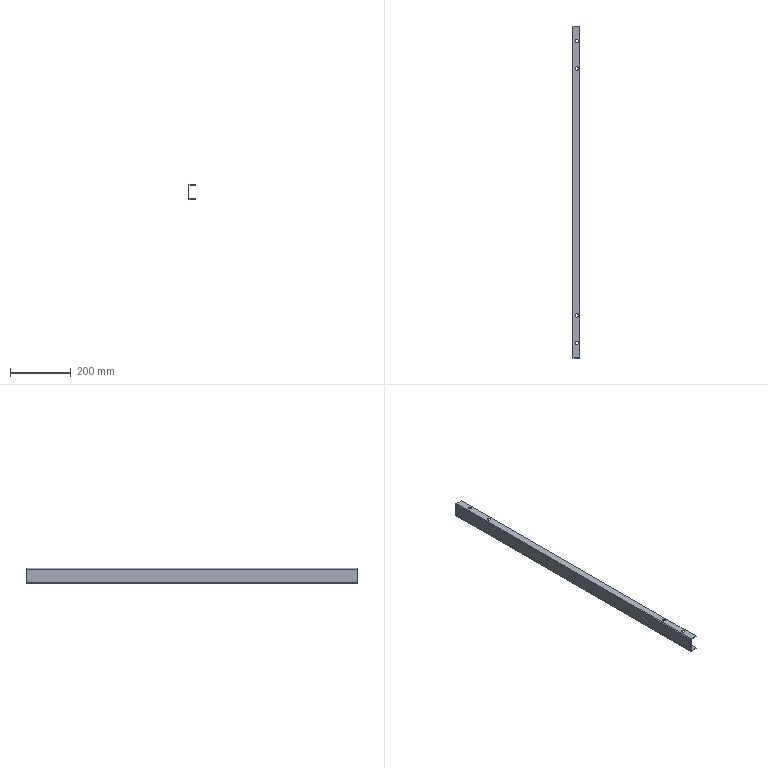Part | SolidWorks | features FlatPattern 1, ICE 1, SMBaseFlange 1, SheetMetal 1 | 1 solid | 38 faces | box 25 x 1095 x 50 mm | volume 206464 mm3 | cylinder 20 | plane 18 | commonest cylinder face diameters 11 x16 0.4 x2 4.4 x2
STEP:
#1=CARTESIAN_POINT('',(20.5,497.5,-23.));
#2=VERTEX_POINT('',#1);
#3=CARTESIAN_POINT('',(9.5,497.5,-23.));
#4=VERTEX_POINT('',#3);
#5=CARTESIAN_POINT('',(15.,497.5,-23.));
#6=DIRECTION('',(0.,0.,-1.));
#7=DIRECTION('',(-1.,0.,0.));
#8=AXIS2_PLACEMENT_3D('',#5,#6,#7);
#9=CIRCLE('',#8,5.5);
#10=EDGE_CURVE('',#2,#4,#9,.T.);
#11=ORIENTED_EDGE('',*,*,#10,.F.);
#12=CARTESIAN_POINT('',(20.5,497.5,-25.));
#13=VERTEX_POINT('',#12);
#14=CARTESIAN_POINT('',(20.5,497.5,25.));
#15=DIRECTION('',(0.,0.,-1.));
#16=VECTOR('',#15,1000.);
#17=LINE('',#14,#16);
#18=EDGE_CURVE('',#2,#13,#17,.T.);
#19=ORIENTED_EDGE('',*,*,#18,.T.);
#20=CARTESIAN_POINT('',(9.5,497.5,-25.));
#21=VERTEX_POINT('',#20);
#22=CARTESIAN_POINT('',(15.,497.5,-25.));
#23=DIRECTION('',(0.,0.,-1.));
#24=DIRECTION('',(-1.,0.,0.));
#25=AXIS2_PLACEMENT_3D('',#22,#23,#24);
#26=CIRCLE('',#25,5.5);
#27=EDGE_CURVE('',#13,#21,#26,.T.);
#28=ORIENTED_EDGE('',*,*,#27,.T.);
#29=CARTESIAN_POINT('',(9.5,497.5,25.));
#30=DIRECTION('',(0.,0.,-1.));
#31=VECTOR('',#30,1000.);
#32=LINE('',#29,#31);
#33=EDGE_CURVE('',#4,#21,#32,.T.);
#34=ORIENTED_EDGE('',*,*,#33,.F.);
#35=EDGE_LOOP('',(#11,#19,#28,#34));
#36=FACE_OUTER_BOUND('',#35,.T.);
#37=CARTESIAN_POINT('',(15.,497.5,25.));
#38=DIRECTION('',(0.,0.,-1.));
#39=DIRECTION('',(-1.,0.,0.));
#40=AXIS2_PLACEMENT_3D('',#37,#38,#39);
#41=CYLINDRICAL_SURFACE('',#40,5.5);
#42=ADVANCED_FACE('',(#36),#41,.F.);
#43=CARTESIAN_POINT('',(20.5,407.5,-23.));
#44=VERTEX_POINT('',#43);
#45=CARTESIAN_POINT('',(9.5,407.5,-23.));
#46=VERTEX_POINT('',#45);
#47=CARTESIAN_POINT('',(15.,407.5,-23.));
#48=DIRECTION('',(0.,0.,-1.));
#49=DIRECTION('',(-1.,0.,0.));
#50=AXIS2_PLACEMENT_3D('',#47,#48,#49);
#51=CIRCLE('',#50,5.5);
#52=EDGE_CURVE('',#44,#46,#51,.T.);
#53=ORIENTED_EDGE('',*,*,#52,.F.);
#54=CARTESIAN_POINT('',(20.5,407.5,-25.));
#55=VERTEX_POINT('',#54);
#56=CARTESIAN_POINT('',(20.5,407.5,25.));
#57=DIRECTION('',(0.,0.,-1.));
#58=VECTOR('',#57,1000.);
#59=LINE('',#56,#58);
#60=EDGE_CURVE('',#44,#55,#59,.T.);
#61=ORIENTED_EDGE('',*,*,#60,.T.);
#62=CARTESIAN_POINT('',(9.5,407.5,-25.));
#63=VERTEX_POINT('',#62);
#64=CARTESIAN_POINT('',(15.,407.5,-25.));
#65=DIRECTION('',(0.,0.,-1.));
#66=DIRECTION('',(-1.,0.,0.));
#67=AXIS2_PLACEMENT_3D('',#64,#65,#66);
#68=CIRCLE('',#67,5.5);
#69=EDGE_CURVE('',#55,#63,#68,.T.);
#70=ORIENTED_EDGE('',*,*,#69,.T.);
#71=CARTESIAN_POINT('',(9.5,407.5,25.));
#72=DIRECTION('',(0.,0.,-1.));
#73=VECTOR('',#72,1000.);
#74=LINE('',#71,#73);
#75=EDGE_CURVE('',#46,#63,#74,.T.);
#76=ORIENTED_EDGE('',*,*,#75,.F.);
#77=EDGE_LOOP('',(#53,#61,#70,#76));
#78=FACE_OUTER_BOUND('',#77,.T.);
#79=CARTESIAN_POINT('',(15.,407.5,25.));
#80=DIRECTION('',(0.,0.,-1.));
#81=DIRECTION('',(-1.,0.,0.));
#82=AXIS2_PLACEMENT_3D('',#79,#80,#81);
#83=CYLINDRICAL_SURFACE('',#82,5.5);
#84=ADVANCED_FACE('',(#78),#83,.F.);
#85=CARTESIAN_POINT('',(20.5,-407.5,-23.));
#86=VERTEX_POINT('',#85);
#87=CARTESIAN_POINT('',(9.5,-407.5,-23.));
#88=VERTEX_POINT('',#87);
#89=CARTESIAN_POINT('',(15.,-407.5,-23.));
#90=DIRECTION('',(0.,0.,-1.));
#91=DIRECTION('',(-1.,0.,0.));
#92=AXIS2_PLACEMENT_3D('',#89,#90,#91);
#93=CIRCLE('',#92,5.5);
#94=EDGE_CURVE('',#86,#88,#93,.T.);
#95=ORIENTED_EDGE('',*,*,#94,.F.);
#96=CARTESIAN_POINT('',(20.5,-407.5,-25.));
#97=VERTEX_POINT('',#96);
#98=CARTESIAN_POINT('',(20.5,-407.5,25.));
#99=DIRECTION('',(0.,0.,-1.));
#100=VECTOR('',#99,1000.);
#101=LINE('',#98,#100);
#102=EDGE_CURVE('',#86,#97,#101,.T.);
#103=ORIENTED_EDGE('',*,*,#102,.T.);
#104=CARTESIAN_POINT('',(9.5,-407.5,-25.));
#105=VERTEX_POINT('',#104);
#106=CARTESIAN_POINT('',(15.,-407.5,-25.));
#107=DIRECTION('',(0.,0.,-1.));
#108=DIRECTION('',(-1.,0.,0.));
#109=AXIS2_PLACEMENT_3D('',#106,#107,#108);
#110=CIRCLE('',#109,5.5);
#111=EDGE_CURVE('',#97,#105,#110,.T.);
#112=ORIENTED_EDGE('',*,*,#111,.T.);
#113=CARTESIAN_POINT('',(9.5,-407.5,25.));
#114=DIRECTION('',(0.,0.,-1.));
#115=VECTOR('',#114,1000.);
#116=LINE('',#113,#115);
#117=EDGE_CURVE('',#88,#105,#116,.T.);
#118=ORIENTED_EDGE('',*,*,#117,.F.);
#119=EDGE_LOOP('',(#95,#103,#112,#118));
#120=FACE_OUTER_BOUND('',#119,.T.);
#121=CARTESIAN_POINT('',(15.,-407.5,25.));
#122=DIRECTION('',(0.,0.,-1.));
#123=DIRECTION('',(-1.,0.,0.));
#124=AXIS2_PLACEMENT_3D('',#121,#122,#123);
#125=CYLINDRICAL_SURFACE('',#124,5.5);
#126=ADVANCED_FACE('',(#120),#125,.F.);
#127=CARTESIAN_POINT('',(20.5,-497.5,-23.));
#128=VERTEX_POINT('',#127);
#129=CARTESIAN_POINT('',(9.5,-497.5,-23.));
#130=VERTEX_POINT('',#129);
#131=CARTESIAN_POINT('',(15.,-497.5,-23.));
#132=DIRECTION('',(0.,0.,-1.));
#133=DIRECTION('',(-1.,0.,0.));
#134=AXIS2_PLACEMENT_3D('',#131,#132,#133);
#135=CIRCLE('',#134,5.5);
#136=EDGE_CURVE('',#128,#130,#135,.T.);
#137=ORIENTED_EDGE('',*,*,#136,.F.);
#138=CARTESIAN_POINT('',(20.5,-497.5,-25.));
#139=VERTEX_POINT('',#138);
#140=CARTESIAN_POINT('',(20.5,-497.5,25.));
#141=DIRECTION('',(0.,0.,-1.));
#142=VECTOR('',#141,1000.);
#143=LINE('',#140,#142);
#144=EDGE_CURVE('',#128,#139,#143,.T.);
#145=ORIENTED_EDGE('',*,*,#144,.T.);
#146=CARTESIAN_POINT('',(9.5,-497.5,-25.));
#147=VERTEX_POINT('',#146);
#148=CARTESIAN_POINT('',(15.,-497.5,-25.));
#149=DIRECTION('',(0.,0.,-1.));
#150=DIRECTION('',(-1.,0.,0.));
#151=AXIS2_PLACEMENT_3D('',#148,#149,#150);
#152=CIRCLE('',#151,5.5);
#153=EDGE_CURVE('',#139,#147,#152,.T.);
#154=ORIENTED_EDGE('',*,*,#153,.T.);
#155=CARTESIAN_POINT('',(9.5,-497.5,25.));
#156=DIRECTION('',(0.,0.,-1.));
#157=VECTOR('',#156,1000.);
#158=LINE('',#155,#157);
#159=EDGE_CURVE('',#130,#147,#158,.T.);
#160=ORIENTED_EDGE('',*,*,#159,.F.);
#161=EDGE_LOOP('',(#137,#145,#154,#160));
#162=FACE_OUTER_BOUND('',#161,.T.);
#163=CARTESIAN_POINT('',(15.,-497.5,25.));
#164=DIRECTION('',(0.,0.,-1.));
#165=DIRECTION('',(-1.,0.,0.));
#166=AXIS2_PLACEMENT_3D('',#163,#164,#165);
#167=CYLINDRICAL_SURFACE('',#166,5.5);
#168=ADVANCED_FACE('',(#162),#167,.F.);
#169=CARTESIAN_POINT('',(20.5,497.5,25.));
#170=VERTEX_POINT('',#169);
#171=CARTESIAN_POINT('',(9.5,497.5,25.));
#172=VERTEX_POINT('',#171);
#173=CARTESIAN_POINT('',(15.,497.5,25.));
#174=DIRECTION('',(0.,0.,-1.));
#175=DIRECTION('',(-1.,0.,0.));
#176=AXIS2_PLACEMENT_3D('',#173,#174,#175);
#177=CIRCLE('',#176,5.5);
#178=EDGE_CURVE('',#170,#172,#177,.T.);
#179=ORIENTED_EDGE('',*,*,#178,.F.);
#180=CARTESIAN_POINT('',(20.5,497.5,23.));
#181=VERTEX_POINT('',#180);
#182=CARTESIAN_POINT('',(20.5,497.5,25.));
#183=DIRECTION('',(0.,0.,-1.));
#184=VECTOR('',#183,1000.);
#185=LINE('',#182,#184);
#186=EDGE_CURVE('',#170,#181,#185,.T.);
#187=ORIENTED_EDGE('',*,*,#186,.T.);
#188=CARTESIAN_POINT('',(9.5,497.5,23.));
#189=VERTEX_POINT('',#188);
#190=CARTESIAN_POINT('',(15.,497.5,23.));
#191=DIRECTION('',(0.,0.,1.));
#192=DIRECTION('',(1.,0.,0.));
#193=AXIS2_PLACEMENT_3D('',#190,#191,#192);
#194=CIRCLE('',#193,5.5);
#195=EDGE_CURVE('',#189,#181,#194,.T.);
#196=ORIENTED_EDGE('',*,*,#195,.F.);
#197=CARTESIAN_POINT('',(9.5,497.5,25.));
#198=DIRECTION('',(0.,0.,-1.));
#199=VECTOR('',#198,1000.);
#200=LINE('',#197,#199);
#201=EDGE_CURVE('',#172,#189,#200,.T.);
#202=ORIENTED_EDGE('',*,*,#201,.F.);
#203=EDGE_LOOP('',(#179,#187,#196,#202));
#204=FACE_OUTER_BOUND('',#203,.T.);
#205=CARTESIAN_POINT('',(15.,497.5,25.));
#206=DIRECTION('',(0.,0.,-1.));
#207=DIRECTION('',(-1.,0.,0.));
#208=AXIS2_PLACEMENT_3D('',#205,#206,#207);
#209=CYLINDRICAL_SURFACE('',#208,5.5);
#210=ADVANCED_FACE('',(#204),#209,.F.);
#211=CARTESIAN_POINT('',(20.5,407.5,25.));
#212=VERTEX_POINT('',#211);
#213=CARTESIAN_POINT('',(9.5,407.5,25.));
#214=VERTEX_POINT('',#213);
#215=CARTESIAN_POINT('',(15.,407.5,25.));
#216=DIRECTION('',(0.,0.,-1.));
#217=DIRECTION('',(-1.,0.,0.));
#218=AXIS2_PLACEMENT_3D('',#215,#216,#217);
#219=CIRCLE('',#218,5.5);
#220=EDGE_CURVE('',#212,#214,#219,.T.);
#221=ORIENTED_EDGE('',*,*,#220,.F.);
#222=CARTESIAN_POINT('',(20.5,407.5,23.));
#223=VERTEX_POINT('',#222);
#224=CARTESIAN_POINT('',(20.5,407.5,25.));
#225=DIRECTION('',(0.,0.,-1.));
#226=VECTOR('',#225,1000.);
#227=LINE('',#224,#226);
#228=EDGE_CURVE('',#212,#223,#227,.T.);
#229=ORIENTED_EDGE('',*,*,#228,.T.);
#230=CARTESIAN_POINT('',(9.5,407.5,23.));
#231=VERTEX_POINT('',#230);
#232=CARTESIAN_POINT('',(15.,407.5,23.));
#233=DIRECTION('',(0.,0.,1.));
#234=DIRECTION('',(1.,0.,0.));
#235=AXIS2_PLACEMENT_3D('',#232,#233,#234);
#236=CIRCLE('',#235,5.5);
#237=EDGE_CURVE('',#231,#223,#236,.T.);
#238=ORIENTED_EDGE('',*,*,#237,.F.);
#239=CARTESIAN_POINT('',(9.5,407.5,25.));
#240=DIRECTION('',(0.,0.,-1.));
#241=VECTOR('',#240,1000.);
#242=LINE('',#239,#241);
#243=EDGE_CURVE('',#214,#231,#242,.T.);
#244=ORIENTED_EDGE('',*,*,#243,.F.);
#245=EDGE_LOOP('',(#221,#229,#238,#244));
#246=FACE_OUTER_BOUND('',#245,.T.);
#247=CARTESIAN_POINT('',(15.,407.5,25.));
#248=DIRECTION('',(0.,0.,-1.));
#249=DIRECTION('',(-1.,0.,0.));
#250=AXIS2_PLACEMENT_3D('',#247,#248,#249);
#251=CYLINDRICAL_SURFACE('',#250,5.5);
#252=ADVANCED_FACE('',(#246),#251,.F.);
#253=CARTESIAN_POINT('',(20.5,-407.5,25.));
#254=VERTEX_POINT('',#253);
#255=CARTESIAN_POINT('',(9.5,-407.5,25.));
#256=VERTEX_POINT('',#255);
#257=CARTESIAN_POINT('',(15.,-407.5,25.));
#258=DIRECTION('',(0.,0.,-1.));
#259=DIRECTION('',(1.,0.,0.));
#260=AXIS2_PLACEMENT_3D('',#257,#258,#259);
#261=CIRCLE('',#260,5.5);
#262=EDGE_CURVE('',#254,#256,#261,.T.);
#263=ORIENTED_EDGE('',*,*,#262,.F.);
#264=CARTESIAN_POINT('',(20.5,-407.5,23.));
#265=VERTEX_POINT('',#264);
#266=CARTESIAN_POINT('',(20.5,-407.5,25.));
#267=DIRECTION('',(0.,0.,-1.));
#268=VECTOR('',#267,1000.);
#269=LINE('',#266,#268);
#270=EDGE_CURVE('',#254,#265,#269,.T.);
#271=ORIENTED_EDGE('',*,*,#270,.T.);
#272=CARTESIAN_POINT('',(9.5,-407.5,23.));
#273=VERTEX_POINT('',#272);
#274=CARTESIAN_POINT('',(15.,-407.5,23.));
#275=DIRECTION('',(0.,0.,1.));
#276=DIRECTION('',(1.,0.,0.));
#277=AXIS2_PLACEMENT_3D('',#274,#275,#276);
#278=CIRCLE('',#277,5.5);
#279=EDGE_CURVE('',#273,#265,#278,.T.);
#280=ORIENTED_EDGE('',*,*,#279,.F.);
#281=CARTESIAN_POINT('',(9.5,-407.5,25.));
#282=DIRECTION('',(0.,0.,-1.));
#283=VECTOR('',#282,1000.);
#284=LINE('',#281,#283);
#285=EDGE_CURVE('',#256,#273,#284,.T.);
#286=ORIENTED_EDGE('',*,*,#285,.F.);
#287=EDGE_LOOP('',(#263,#271,#280,#286));
#288=FACE_OUTER_BOUND('',#287,.T.);
#289=CARTESIAN_POINT('',(15.,-407.5,25.));
#290=DIRECTION('',(0.,0.,-1.));
#291=DIRECTION('',(-1.,0.,0.));
#292=AXIS2_PLACEMENT_3D('',#289,#290,#291);
#293=CYLINDRICAL_SURFACE('',#292,5.5);
#294=ADVANCED_FACE('',(#288),#293,.F.);
#295=CARTESIAN_POINT('',(20.5,-497.5,25.));
#296=VERTEX_POINT('',#295);
#297=CARTESIAN_POINT('',(9.5,-497.5,25.));
#298=VERTEX_POINT('',#297);
#299=CARTESIAN_POINT('',(15.,-497.5,25.));
#300=DIRECTION('',(0.,0.,-1.));
#301=DIRECTION('',(1.,0.,0.));
#302=AXIS2_PLACEMENT_3D('',#299,#300,#301);
#303=CIRCLE('',#302,5.5);
#304=EDGE_CURVE('',#296,#298,#303,.T.);
#305=ORIENTED_EDGE('',*,*,#304,.F.);
#306=CARTESIAN_POINT('',(20.5,-497.5,23.));
#307=VERTEX_POINT('',#306);
#308=CARTESIAN_POINT('',(20.5,-497.5,25.));
#309=DIRECTION('',(0.,0.,-1.));
#310=VECTOR('',#309,1000.);
#311=LINE('',#308,#310);
#312=EDGE_CURVE('',#296,#307,#311,.T.);
#313=ORIENTED_EDGE('',*,*,#312,.T.);
#314=CARTESIAN_POINT('',(9.5,-497.5,23.));
#315=VERTEX_POINT('',#314);
#316=CARTESIAN_POINT('',(15.,-497.5,23.));
#317=DIRECTION('',(0.,0.,1.));
#318=DIRECTION('',(1.,0.,0.));
#319=AXIS2_PLACEMENT_3D('',#316,#317,#318);
#320=CIRCLE('',#319,5.5);
#321=EDGE_CURVE('',#315,#307,#320,.T.);
#322=ORIENTED_EDGE('',*,*,#321,.F.);
#323=CARTESIAN_POINT('',(9.5,-497.5,25.));
#324=DIRECTION('',(0.,0.,-1.));
#325=VECTOR('',#324,1000.);
#326=LINE('',#323,#325);
#327=EDGE_CURVE('',#298,#315,#326,.T.);
#328=ORIENTED_EDGE('',*,*,#327,.F.);
#329=EDGE_LOOP('',(#305,#313,#322,#328));
#330=FACE_OUTER_BOUND('',#329,.T.);
#331=CARTESIAN_POINT('',(15.,-497.5,25.));
#332=DIRECTION('',(0.,0.,-1.));
#333=DIRECTION('',(-1.,0.,0.));
#334=AXIS2_PLACEMENT_3D('',#331,#332,#333);
#335=CYLINDRICAL_SURFACE('',#334,5.5);
#336=ADVANCED_FACE('',(#330),#335,.F.);
#337=CARTESIAN_POINT('',(0.,547.5,22.8));
#338=VERTEX_POINT('',#337);
#339=CARTESIAN_POINT('',(2.,547.5,22.8));
#340=VERTEX_POINT('',#339);
#341=CARTESIAN_POINT('',(0.,547.5,22.8));
#342=DIRECTION('',(1.,0.,0.));
#343=VECTOR('',#342,1000.);
#344=LINE('',#341,#343);
#345=EDGE_CURVE('',#338,#340,#344,.T.);
#346=ORIENTED_EDGE('',*,*,#345,.F.);
#347=CARTESIAN_POINT('',(2.2,547.5,25.));
#348=VERTEX_POINT('',#347);
#349=CARTESIAN_POINT('',(2.2,547.5,22.8));
#350=DIRECTION('',(0.,-1.,0.));
#351=DIRECTION('',(0.,0.,1.));
#352=AXIS2_PLACEMENT_3D('',#349,#350,#351);
#353=CIRCLE('',#352,2.2);
#354=EDGE_CURVE('',#348,#338,#353,.T.);
#355=ORIENTED_EDGE('',*,*,#354,.F.);
#356=CARTESIAN_POINT('',(2.2,547.5,23.));
#357=VERTEX_POINT('',#356);
#358=CARTESIAN_POINT('',(2.2,547.5,23.));
#359=DIRECTION('',(0.,0.,1.));
#360=VECTOR('',#359,1000.);
#361=LINE('',#358,#360);
#362=EDGE_CURVE('',#357,#348,#361,.T.);
#363=ORIENTED_EDGE('',*,*,#362,.F.);
#364=CARTESIAN_POINT('',(2.2,547.5,22.8));
#365=DIRECTION('',(0.,-1.,0.));
#366=DIRECTION('',(1.,0.,0.));
#367=AXIS2_PLACEMENT_3D('',#364,#365,#366);
#368=CIRCLE('',#367,0.2);
#369=EDGE_CURVE('',#357,#340,#368,.T.);
#370=ORIENTED_EDGE('',*,*,#369,.T.);
#371=EDGE_LOOP('',(#346,#355,#363,#370));
#372=FACE_OUTER_BOUND('',#371,.T.);
#373=CARTESIAN_POINT('',(0.,547.5,22.8));
#374=DIRECTION('',(0.,1.,0.));
#375=DIRECTION('',(0.,0.,1.));
#376=AXIS2_PLACEMENT_3D('',#373,#374,#375);
#377=PLANE('',#376);
#378=ADVANCED_FACE('',(#372),#377,.T.);
#379=CARTESIAN_POINT('',(0.,547.5,-22.8));
#380=VERTEX_POINT('',#379);
#381=CARTESIAN_POINT('',(0.,547.5,-25.));
#382=DIRECTION('',(0.,0.,-1.));
#383=VECTOR('',#382,1000.);
#384=LINE('',#381,#383);
#385=EDGE_CURVE('',#338,#380,#384,.T.);
#386=ORIENTED_EDGE('',*,*,#385,.F.);
#387=ORIENTED_EDGE('',*,*,#345,.T.);
#388=CARTESIAN_POINT('',(2.,547.5,-22.8));
#389=VERTEX_POINT('',#388);
#390=CARTESIAN_POINT('',(2.,547.5,-25.));
#391=DIRECTION('',(0.,0.,-1.));
#392=VECTOR('',#391,1000.);
#393=LINE('',#390,#392);
#394=EDGE_CURVE('',#340,#389,#393,.T.);
#395=ORIENTED_EDGE('',*,*,#394,.T.);
#396=CARTESIAN_POINT('',(2.,547.5,-22.8));
#397=DIRECTION('',(-1.,0.,0.));
#398=VECTOR('',#397,1000.);
#399=LINE('',#396,#398);
#400=EDGE_CURVE('',#389,#380,#399,.T.);
#401=ORIENTED_EDGE('',*,*,#400,.T.);
#402=EDGE_LOOP('',(#386,#387,#395,#401));
#403=FACE_OUTER_BOUND('',#402,.T.);
#404=CARTESIAN_POINT('',(2.2,547.5,23.));
#405=DIRECTION('',(0.,1.,0.));
#406=DIRECTION('',(0.,0.,1.));
#407=AXIS2_PLACEMENT_3D('',#404,#405,#406);
#408=PLANE('',#407);
#409=ADVANCED_FACE('',(#403),#408,.T.);
#410=CARTESIAN_POINT('',(2.2,-547.5,25.));
#411=VERTEX_POINT('',#410);
#412=CARTESIAN_POINT('',(2.2,-547.5,23.));
#413=VERTEX_POINT('',#412);
#414=CARTESIAN_POINT('',(2.2,-547.5,25.));
#415=DIRECTION('',(0.,0.,-1.));
#416=VECTOR('',#415,1000.);
#417=LINE('',#414,#416);
#418=EDGE_CURVE('',#411,#413,#417,.T.);
#419=ORIENTED_EDGE('',*,*,#418,.F.);
#420=CARTESIAN_POINT('',(0.,-547.5,22.8));
#421=VERTEX_POINT('',#420);
#422=CARTESIAN_POINT('',(2.2,-547.5,22.8));
#423=DIRECTION('',(0.,-1.,0.));
#424=DIRECTION('',(0.,0.,1.));
#425=AXIS2_PLACEMENT_3D('',#422,#423,#424);
#426=CIRCLE('',#425,2.2);
#427=EDGE_CURVE('',#411,#421,#426,.T.);
#428=ORIENTED_EDGE('',*,*,#427,.T.);
#429=CARTESIAN_POINT('',(2.,-547.5,22.8));
#430=VERTEX_POINT('',#429);
#431=CARTESIAN_POINT('',(2.,-547.5,22.8));
#432=DIRECTION('',(-1.,0.,0.));
#433=VECTOR('',#432,1000.);
#434=LINE('',#431,#433);
#435=EDGE_CURVE('',#430,#421,#434,.T.);
#436=ORIENTED_EDGE('',*,*,#435,.F.);
#437=CARTESIAN_POINT('',(2.2,-547.5,22.8));
#438=DIRECTION('',(0.,-1.,0.));
#439=DIRECTION('',(1.,0.,0.));
#440=AXIS2_PLACEMENT_3D('',#437,#438,#439);
#441=CIRCLE('',#440,0.2);
#442=EDGE_CURVE('',#413,#430,#441,.T.);
#443=ORIENTED_EDGE('',*,*,#442,.F.);
#444=EDGE_LOOP('',(#419,#428,#436,#443));
#445=FACE_OUTER_BOUND('',#444,.T.);
#446=CARTESIAN_POINT('',(2.2,-547.5,25.));
#447=DIRECTION('',(0.,-1.,0.));
#448=DIRECTION('',(0.,0.,-1.));
#449=AXIS2_PLACEMENT_3D('',#446,#447,#448);
#450=PLANE('',#449);
#451=ADVANCED_FACE('',(#445),#450,.T.);
#452=CARTESIAN_POINT('',(25.,-547.5,25.));
#453=VERTEX_POINT('',#452);
#454=CARTESIAN_POINT('',(0.,-547.5,25.));
#455=DIRECTION('',(-1.,0.,0.));
#456=VECTOR('',#455,1000.);
#457=LINE('',#454,#456);
#458=EDGE_CURVE('',#453,#411,#457,.T.);
#459=ORIENTED_EDGE('',*,*,#458,.T.);
#460=ORIENTED_EDGE('',*,*,#418,.T.);
#461=CARTESIAN_POINT('',(25.,-547.5,23.));
#462=VERTEX_POINT('',#461);
#463=CARTESIAN_POINT('',(0.,-547.5,23.));
#464=DIRECTION('',(-1.,0.,0.));
#465=VECTOR('',#464,1000.);
#466=LINE('',#463,#465);
#467=EDGE_CURVE('',#462,#413,#466,.T.);
#468=ORIENTED_EDGE('',*,*,#467,.F.);
#469=CARTESIAN_POINT('',(25.,-547.5,23.));
#470=DIRECTION('',(0.,0.,1.));
#471=VECTOR('',#470,1000.);
#472=LINE('',#469,#471);
#473=EDGE_CURVE('',#462,#453,#472,.T.);
#474=ORIENTED_EDGE('',*,*,#473,.T.);
#475=EDGE_LOOP('',(#459,#460,#468,#474));
#476=FACE_OUTER_BOUND('',#475,.T.);
#477=CARTESIAN_POINT('',(2.,-547.5,22.8));
#478=DIRECTION('',(0.,-1.,0.));
#479=DIRECTION('',(0.,0.,-1.));
#480=AXIS2_PLACEMENT_3D('',#477,#478,#479);
#481=PLANE('',#480);
#482=ADVANCED_FACE('',(#476),#481,.T.);
#483=CARTESIAN_POINT('',(2.2,547.5,-25.));
#484=VERTEX_POINT('',#483);
#485=CARTESIAN_POINT('',(2.2,547.5,-23.));
#486=VERTEX_POINT('',#485);
#487=CARTESIAN_POINT('',(2.2,547.5,-25.));
#488=DIRECTION('',(0.,0.,1.));
#489=VECTOR('',#488,1000.);
#490=LINE('',#487,#489);
#491=EDGE_CURVE('',#484,#486,#490,.T.);
#492=ORIENTED_EDGE('',*,*,#491,.F.);
#493=CARTESIAN_POINT('',(2.2,547.5,-22.8));
#494=DIRECTION('',(0.,-1.,0.));
#495=DIRECTION('',(0.,0.,1.));
#496=AXIS2_PLACEMENT_3D('',#493,#494,#495);
#497=CIRCLE('',#496,2.2);
#498=EDGE_CURVE('',#380,#484,#497,.T.);
#499=ORIENTED_EDGE('',*,*,#498,.F.);
#500=ORIENTED_EDGE('',*,*,#400,.F.);
#501=CARTESIAN_POINT('',(2.2,547.5,-22.8));
#502=DIRECTION('',(0.,-1.,0.));
#503=DIRECTION('',(1.,0.,0.));
#504=AXIS2_PLACEMENT_3D('',#501,#502,#503);
#505=CIRCLE('',#504,0.2);
#506=EDGE_CURVE('',#389,#486,#505,.T.);
#507=ORIENTED_EDGE('',*,*,#506,.T.);
#508=EDGE_LOOP('',(#492,#499,#500,#507));
#509=FACE_OUTER_BOUND('',#508,.T.);
#510=CARTESIAN_POINT('',(2.2,547.5,-25.));
#511=DIRECTION('',(0.,1.,0.));
#512=DIRECTION('',(0.,0.,1.));
#513=AXIS2_PLACEMENT_3D('',#510,#511,#512);
#514=PLANE('',#513);
#515=ADVANCED_FACE('',(#509),#514,.T.);
#516=CARTESIAN_POINT('',(25.,547.5,-25.));
#517=VERTEX_POINT('',#516);
#518=CARTESIAN_POINT('',(0.,547.5,-25.));
#519=DIRECTION('',(1.,0.,0.));
#520=VECTOR('',#519,1000.);
#521=LINE('',#518,#520);
#522=EDGE_CURVE('',#484,#517,#521,.T.);
#523=ORIENTED_EDGE('',*,*,#522,.F.);
#524=ORIENTED_EDGE('',*,*,#491,.T.);
#525=CARTESIAN_POINT('',(25.,547.5,-23.));
#526=VERTEX_POINT('',#525);
#527=CARTESIAN_POINT('',(0.,547.5,-23.));
#528=DIRECTION('',(1.,0.,0.));
#529=VECTOR('',#528,1000.);
#530=LINE('',#527,#529);
#531=EDGE_CURVE('',#486,#526,#530,.T.);
#532=ORIENTED_EDGE('',*,*,#531,.T.);
#533=CARTESIAN_POINT('',(25.,547.5,-25.));
#534=DIRECTION('',(0.,0.,1.));
#535=VECTOR('',#534,1000.);
#536=LINE('',#533,#535);
#537=EDGE_CURVE('',#517,#526,#536,.T.);
#538=ORIENTED_EDGE('',*,*,#537,.F.);
#539=EDGE_LOOP('',(#523,#524,#532,#538));
#540=FACE_OUTER_BOUND('',#539,.T.);
#541=CARTESIAN_POINT('',(2.,547.5,-22.8));
#542=DIRECTION('',(0.,1.,0.));
#543=DIRECTION('',(0.,0.,1.));
#544=AXIS2_PLACEMENT_3D('',#541,#542,#543);
#545=PLANE('',#544);
#546=ADVANCED_FACE('',(#540),#545,.T.);
#547=CARTESIAN_POINT('',(0.,-547.5,-22.8));
#548=VERTEX_POINT('',#547);
#549=CARTESIAN_POINT('',(2.,-547.5,-22.8));
#550=VERTEX_POINT('',#549);
#551=CARTESIAN_POINT('',(0.,-547.5,-22.8));
#552=DIRECTION('',(1.,0.,0.));
#553=VECTOR('',#552,1000.);
#554=LINE('',#551,#553);
#555=EDGE_CURVE('',#548,#550,#554,.T.);
#556=ORIENTED_EDGE('',*,*,#555,.F.);
#557=CARTESIAN_POINT('',(2.2,-547.5,-25.));
#558=VERTEX_POINT('',#557);
#559=CARTESIAN_POINT('',(2.2,-547.5,-22.8));
#560=DIRECTION('',(0.,-1.,0.));
#561=DIRECTION('',(0.,0.,1.));
#562=AXIS2_PLACEMENT_3D('',#559,#560,#561);
#563=CIRCLE('',#562,2.2);
#564=EDGE_CURVE('',#548,#558,#563,.T.);
#565=ORIENTED_EDGE('',*,*,#564,.T.);
#566=CARTESIAN_POINT('',(2.2,-547.5,-23.));
#567=VERTEX_POINT('',#566);
#568=CARTESIAN_POINT('',(2.2,-547.5,-23.));
#569=DIRECTION('',(0.,0.,-1.));
#570=VECTOR('',#569,1000.);
#571=LINE('',#568,#570);
#572=EDGE_CURVE('',#567,#558,#571,.T.);
#573=ORIENTED_EDGE('',*,*,#572,.F.);
#574=CARTESIAN_POINT('',(2.2,-547.5,-22.8));
#575=DIRECTION('',(0.,-1.,0.));
#576=DIRECTION('',(1.,0.,0.));
#577=AXIS2_PLACEMENT_3D('',#574,#575,#576);
#578=CIRCLE('',#577,0.2);
#579=EDGE_CURVE('',#550,#567,#578,.T.);
#580=ORIENTED_EDGE('',*,*,#579,.F.);
#581=EDGE_LOOP('',(#556,#565,#573,#580));
#582=FACE_OUTER_BOUND('',#581,.T.);
#583=CARTESIAN_POINT('',(0.,-547.5,-22.8));
#584=DIRECTION('',(0.,-1.,0.));
#585=DIRECTION('',(0.,0.,-1.));
#586=AXIS2_PLACEMENT_3D('',#583,#584,#585);
#587=PLANE('',#586);
#588=ADVANCED_FACE('',(#582),#587,.T.);
#589=CARTESIAN_POINT('',(0.,-547.5,-25.));
#590=DIRECTION('',(0.,0.,-1.));
#591=VECTOR('',#590,1000.);
#592=LINE('',#589,#591);
#593=EDGE_CURVE('',#421,#548,#592,.T.);
#594=ORIENTED_EDGE('',*,*,#593,.T.);
#595=ORIENTED_EDGE('',*,*,#555,.T.);
#596=CARTESIAN_POINT('',(2.,-547.5,-25.));
#597=DIRECTION('',(0.,0.,-1.));
#598=VECTOR('',#597,1000.);
#599=LINE('',#596,#598);
#600=EDGE_CURVE('',#430,#550,#599,.T.);
#601=ORIENTED_EDGE('',*,*,#600,.F.);
#602=ORIENTED_EDGE('',*,*,#435,.T.);
#603=EDGE_LOOP('',(#594,#595,#601,#602));
#604=FACE_OUTER_BOUND('',#603,.T.);
#605=CARTESIAN_POINT('',(2.2,-547.5,-23.));
#606=DIRECTION('',(0.,-1.,0.));
#607=DIRECTION('',(0.,0.,-1.));
#608=AXIS2_PLACEMENT_3D('',#605,#606,#607);
#609=PLANE('',#608);
#610=ADVANCED_FACE('',(#604),#609,.T.);
#611=CARTESIAN_POINT('',(15.,497.5,-23.));
#612=DIRECTION('',(0.,0.,-1.));
#613=DIRECTION('',(-1.,0.,0.));
#614=AXIS2_PLACEMENT_3D('',#611,#612,#613);
#615=CIRCLE('',#614,5.5);
#616=EDGE_CURVE('',#4,#2,#615,.T.);
#617=ORIENTED_EDGE('',*,*,#616,.T.);
#618=ORIENTED_EDGE('',*,*,#10,.T.);
#619=EDGE_LOOP('',(#617,#618));
#620=FACE_BOUND('',#619,.T.);
#621=CARTESIAN_POINT('',(15.,407.5,-23.));
#622=DIRECTION('',(0.,0.,-1.));
#623=DIRECTION('',(-1.,0.,0.));
#624=AXIS2_PLACEMENT_3D('',#621,#622,#623);
#625=CIRCLE('',#624,5.5);
#626=EDGE_CURVE('',#46,#44,#625,.T.);
#627=ORIENTED_EDGE('',*,*,#626,.T.);
#628=ORIENTED_EDGE('',*,*,#52,.T.);
#629=EDGE_LOOP('',(#627,#628));
#630=FACE_BOUND('',#629,.T.);
#631=CARTESIAN_POINT('',(15.,-407.5,-23.));
#632=DIRECTION('',(0.,0.,-1.));
#633=DIRECTION('',(-1.,0.,0.));
#634=AXIS2_PLACEMENT_3D('',#631,#632,#633);
#635=CIRCLE('',#634,5.5);
#636=EDGE_CURVE('',#88,#86,#635,.T.);
#637=ORIENTED_EDGE('',*,*,#636,.T.);
#638=ORIENTED_EDGE('',*,*,#94,.T.);
#639=EDGE_LOOP('',(#637,#638));
#640=FACE_BOUND('',#639,.T.);
#641=CARTESIAN_POINT('',(15.,-497.5,-23.));
#642=DIRECTION('',(0.,0.,-1.));
#643=DIRECTION('',(-1.,0.,0.));
#644=AXIS2_PLACEMENT_3D('',#641,#642,#643);
#645=CIRCLE('',#644,5.5);
#646=EDGE_CURVE('',#130,#128,#645,.T.);
#647=ORIENTED_EDGE('',*,*,#646,.T.);
#648=ORIENTED_EDGE('',*,*,#136,.T.);
#649=EDGE_LOOP('',(#647,#648));
#650=FACE_BOUND('',#649,.T.);
#651=CARTESIAN_POINT('',(25.,-547.5,-23.));
#652=VERTEX_POINT('',#651);
#653=CARTESIAN_POINT('',(0.,-547.5,-23.));
#654=DIRECTION('',(1.,0.,0.));
#655=VECTOR('',#654,1000.);
#656=LINE('',#653,#655);
#657=EDGE_CURVE('',#567,#652,#656,.T.);
#658=ORIENTED_EDGE('',*,*,#657,.T.);
#659=CARTESIAN_POINT('',(25.,547.5,-23.));
#660=DIRECTION('',(0.,-1.,0.));
#661=VECTOR('',#660,1000.);
#662=LINE('',#659,#661);
#663=EDGE_CURVE('',#526,#652,#662,.T.);
#664=ORIENTED_EDGE('',*,*,#663,.F.);
#665=ORIENTED_EDGE('',*,*,#531,.F.);
#666=CARTESIAN_POINT('',(2.2,547.5,-23.));
#667=DIRECTION('',(0.,-1.,0.));
#668=VECTOR('',#667,1000.);
#669=LINE('',#666,#668);
#670=EDGE_CURVE('',#486,#567,#669,.T.);
#671=ORIENTED_EDGE('',*,*,#670,.T.);
#672=EDGE_LOOP('',(#658,#664,#665,#671));
#673=FACE_OUTER_BOUND('',#672,.T.);
#674=CARTESIAN_POINT('',(0.,547.5,-23.));
#675=DIRECTION('',(0.,0.,-1.));
#676=DIRECTION('',(-1.,0.,0.));
#677=AXIS2_PLACEMENT_3D('',#674,#675,#676);
#678=PLANE('',#677);
#679=ADVANCED_FACE('',(#620,#630,#640,#650,#673),#678,.F.);
#680=CARTESIAN_POINT('',(25.,-547.5,-25.));
#681=VERTEX_POINT('',#680);
#682=CARTESIAN_POINT('',(25.,-547.5,-25.));
#683=DIRECTION('',(0.,0.,1.));
#684=VECTOR('',#683,1000.);
#685=LINE('',#682,#684);
#686=EDGE_CURVE('',#681,#652,#685,.T.);
#687=ORIENTED_EDGE('',*,*,#686,.F.);
#688=CARTESIAN_POINT('',(25.,547.5,-25.));
#689=DIRECTION('',(0.,-1.,0.));
#690=VECTOR('',#689,1000.);
#691=LINE('',#688,#690);
#692=EDGE_CURVE('',#517,#681,#691,.T.);
#693=ORIENTED_EDGE('',*,*,#692,.F.);
#694=ORIENTED_EDGE('',*,*,#537,.T.);
#695=ORIENTED_EDGE('',*,*,#663,.T.);
#696=EDGE_LOOP('',(#687,#693,#694,#695));
#697=FACE_OUTER_BOUND('',#696,.T.);
#698=CARTESIAN_POINT('',(25.,547.5,-25.));
#699=DIRECTION('',(1.,0.,0.));
#700=DIRECTION('',(0.,0.,-1.));
#701=AXIS2_PLACEMENT_3D('',#698,#699,#700);
#702=PLANE('',#701);
#703=ADVANCED_FACE('',(#697),#702,.T.);
#704=CARTESIAN_POINT('',(15.,497.5,-25.));
#705=DIRECTION('',(0.,0.,-1.));
#706=DIRECTION('',(-1.,0.,0.));
#707=AXIS2_PLACEMENT_3D('',#704,#705,#706);
#708=CIRCLE('',#707,5.5);
#709=EDGE_CURVE('',#21,#13,#708,.T.);
#710=ORIENTED_EDGE('',*,*,#709,.F.);
#711=ORIENTED_EDGE('',*,*,#27,.F.);
#712=EDGE_LOOP('',(#710,#711));
#713=FACE_BOUND('',#712,.T.);
#714=CARTESIAN_POINT('',(15.,407.5,-25.));
#715=DIRECTION('',(0.,0.,-1.));
#716=DIRECTION('',(-1.,0.,0.));
#717=AXIS2_PLACEMENT_3D('',#714,#715,#716);
#718=CIRCLE('',#717,5.5);
#719=EDGE_CURVE('',#63,#55,#718,.T.);
#720=ORIENTED_EDGE('',*,*,#719,.F.);
#721=ORIENTED_EDGE('',*,*,#69,.F.);
#722=EDGE_LOOP('',(#720,#721));
#723=FACE_BOUND('',#722,.T.);
#724=CARTESIAN_POINT('',(15.,-407.5,-25.));
#725=DIRECTION('',(0.,0.,-1.));
#726=DIRECTION('',(-1.,0.,0.));
#727=AXIS2_PLACEMENT_3D('',#724,#725,#726);
#728=CIRCLE('',#727,5.5);
#729=EDGE_CURVE('',#105,#97,#728,.T.);
#730=ORIENTED_EDGE('',*,*,#729,.F.);
#731=ORIENTED_EDGE('',*,*,#111,.F.);
#732=EDGE_LOOP('',(#730,#731));
#733=FACE_BOUND('',#732,.T.);
#734=CARTESIAN_POINT('',(15.,-497.5,-25.));
#735=DIRECTION('',(0.,0.,-1.));
#736=DIRECTION('',(-1.,0.,0.));
#737=AXIS2_PLACEMENT_3D('',#734,#735,#736);
#738=CIRCLE('',#737,5.5);
#739=EDGE_CURVE('',#147,#139,#738,.T.);
#740=ORIENTED_EDGE('',*,*,#739,.F.);
#741=ORIENTED_EDGE('',*,*,#153,.F.);
#742=EDGE_LOOP('',(#740,#741));
#743=FACE_BOUND('',#742,.T.);
#744=CARTESIAN_POINT('',(0.,-547.5,-25.));
#745=DIRECTION('',(1.,0.,0.));
#746=VECTOR('',#745,1000.);
#747=LINE('',#744,#746);
#748=EDGE_CURVE('',#558,#681,#747,.T.);
#749=ORIENTED_EDGE('',*,*,#748,.F.);
#750=CARTESIAN_POINT('',(2.2,547.5,-25.));
#751=DIRECTION('',(0.,-1.,0.));
#752=VECTOR('',#751,1000.);
#753=LINE('',#750,#752);
#754=EDGE_CURVE('',#484,#558,#753,.T.);
#755=ORIENTED_EDGE('',*,*,#754,.F.);
#756=ORIENTED_EDGE('',*,*,#522,.T.);
#757=ORIENTED_EDGE('',*,*,#692,.T.);
#758=EDGE_LOOP('',(#749,#755,#756,#757));
#759=FACE_OUTER_BOUND('',#758,.T.);
#760=CARTESIAN_POINT('',(0.,547.5,-25.));
#761=DIRECTION('',(0.,0.,-1.));
#762=DIRECTION('',(-1.,0.,0.));
#763=AXIS2_PLACEMENT_3D('',#760,#761,#762);
#764=PLANE('',#763);
#765=ADVANCED_FACE('',(#713,#723,#733,#743,#759),#764,.T.);
#766=ORIENTED_EDGE('',*,*,#564,.F.);
#767=CARTESIAN_POINT('',(0.,547.5,-22.8));
#768=DIRECTION('',(0.,-1.,0.));
#769=VECTOR('',#768,1000.);
#770=LINE('',#767,#769);
#771=EDGE_CURVE('',#380,#548,#770,.T.);
#772=ORIENTED_EDGE('',*,*,#771,.F.);
#773=ORIENTED_EDGE('',*,*,#498,.T.);
#774=ORIENTED_EDGE('',*,*,#754,.T.);
#775=EDGE_LOOP('',(#766,#772,#773,#774));
#776=FACE_OUTER_BOUND('',#775,.T.);
#777=CARTESIAN_POINT('',(2.2,547.5,-22.8));
#778=DIRECTION('',(0.,-1.,0.));
#779=DIRECTION('',(0.,0.,-1.));
#780=AXIS2_PLACEMENT_3D('',#777,#778,#779);
#781=CYLINDRICAL_SURFACE('',#780,2.2);
#782=ADVANCED_FACE('',(#776),#781,.T.);
#783=ORIENTED_EDGE('',*,*,#593,.F.);
#784=CARTESIAN_POINT('',(0.,547.5,22.8));
#785=DIRECTION('',(0.,-1.,0.));
#786=VECTOR('',#785,1000.);
#787=LINE('',#784,#786);
#788=EDGE_CURVE('',#338,#421,#787,.T.);
#789=ORIENTED_EDGE('',*,*,#788,.F.);
#790=ORIENTED_EDGE('',*,*,#385,.T.);
#791=ORIENTED_EDGE('',*,*,#771,.T.);
#792=EDGE_LOOP('',(#783,#789,#790,#791));
#793=FACE_OUTER_BOUND('',#792,.T.);
#794=CARTESIAN_POINT('',(0.,547.5,-25.));
#795=DIRECTION('',(-1.,0.,0.));
#796=DIRECTION('',(0.,0.,1.));
#797=AXIS2_PLACEMENT_3D('',#794,#795,#796);
#798=PLANE('',#797);
#799=ADVANCED_FACE('',(#793),#798,.T.);
#800=ORIENTED_EDGE('',*,*,#427,.F.);
#801=CARTESIAN_POINT('',(2.2,547.5,25.));
#802=DIRECTION('',(0.,-1.,0.));
#803=VECTOR('',#802,1000.);
#804=LINE('',#801,#803);
#805=EDGE_CURVE('',#348,#411,#804,.T.);
#806=ORIENTED_EDGE('',*,*,#805,.F.);
#807=ORIENTED_EDGE('',*,*,#354,.T.);
#808=ORIENTED_EDGE('',*,*,#788,.T.);
#809=EDGE_LOOP('',(#800,#806,#807,#808));
#810=FACE_OUTER_BOUND('',#809,.T.);
#811=CARTESIAN_POINT('',(2.2,547.5,22.8));
#812=DIRECTION('',(0.,-1.,0.));
#813=DIRECTION('',(0.,0.,-1.));
#814=AXIS2_PLACEMENT_3D('',#811,#812,#813);
#815=CYLINDRICAL_SURFACE('',#814,2.2);
#816=ADVANCED_FACE('',(#810),#815,.T.);
#817=CARTESIAN_POINT('',(15.,497.5,25.));
#818=DIRECTION('',(0.,0.,-1.));
#819=DIRECTION('',(-1.,0.,0.));
#820=AXIS2_PLACEMENT_3D('',#817,#818,#819);
#821=CIRCLE('',#820,5.5);
#822=EDGE_CURVE('',#172,#170,#821,.T.);
#823=ORIENTED_EDGE('',*,*,#822,.T.);
#824=ORIENTED_EDGE('',*,*,#178,.T.);
#825=EDGE_LOOP('',(#823,#824));
#826=FACE_BOUND('',#825,.T.);
#827=CARTESIAN_POINT('',(15.,407.5,25.));
#828=DIRECTION('',(0.,0.,-1.));
#829=DIRECTION('',(-1.,0.,0.));
#830=AXIS2_PLACEMENT_3D('',#827,#828,#829);
#831=CIRCLE('',#830,5.5);
#832=EDGE_CURVE('',#214,#212,#831,.T.);
#833=ORIENTED_EDGE('',*,*,#832,.T.);
#834=ORIENTED_EDGE('',*,*,#220,.T.);
#835=EDGE_LOOP('',(#833,#834));
#836=FACE_BOUND('',#835,.T.);
#837=CARTESIAN_POINT('',(15.,-407.5,25.));
#838=DIRECTION('',(0.,0.,-1.));
#839=DIRECTION('',(1.,0.,0.));
#840=AXIS2_PLACEMENT_3D('',#837,#838,#839);
#841=CIRCLE('',#840,5.5);
#842=EDGE_CURVE('',#256,#254,#841,.T.);
#843=ORIENTED_EDGE('',*,*,#842,.T.);
#844=ORIENTED_EDGE('',*,*,#262,.T.);
#845=EDGE_LOOP('',(#843,#844));
#846=FACE_BOUND('',#845,.T.);
#847=CARTESIAN_POINT('',(15.,-497.5,25.));
#848=DIRECTION('',(0.,0.,-1.));
#849=DIRECTION('',(1.,0.,0.));
#850=AXIS2_PLACEMENT_3D('',#847,#848,#849);
#851=CIRCLE('',#850,5.5);
#852=EDGE_CURVE('',#298,#296,#851,.T.);
#853=ORIENTED_EDGE('',*,*,#852,.T.);
#854=ORIENTED_EDGE('',*,*,#304,.T.);
#855=EDGE_LOOP('',(#853,#854));
#856=FACE_BOUND('',#855,.T.);
#857=ORIENTED_EDGE('',*,*,#458,.F.);
#858=CARTESIAN_POINT('',(25.,547.5,25.));
#859=VERTEX_POINT('',#858);
#860=CARTESIAN_POINT('',(25.,547.5,25.));
#861=DIRECTION('',(0.,-1.,0.));
#862=VECTOR('',#861,1000.);
#863=LINE('',#860,#862);
#864=EDGE_CURVE('',#859,#453,#863,.T.);
#865=ORIENTED_EDGE('',*,*,#864,.F.);
#866=CARTESIAN_POINT('',(0.,547.5,25.));
#867=DIRECTION('',(-1.,0.,0.));
#868=VECTOR('',#867,1000.);
#869=LINE('',#866,#868);
#870=EDGE_CURVE('',#859,#348,#869,.T.);
#871=ORIENTED_EDGE('',*,*,#870,.T.);
#872=ORIENTED_EDGE('',*,*,#805,.T.);
#873=EDGE_LOOP('',(#857,#865,#871,#872));
#874=FACE_OUTER_BOUND('',#873,.T.);
#875=CARTESIAN_POINT('',(0.,547.5,25.));
#876=DIRECTION('',(0.,0.,1.));
#877=DIRECTION('',(1.,0.,0.));
#878=AXIS2_PLACEMENT_3D('',#875,#876,#877);
#879=PLANE('',#878);
#880=ADVANCED_FACE('',(#826,#836,#846,#856,#874),#879,.T.);
#881=ORIENTED_EDGE('',*,*,#473,.F.);
#882=CARTESIAN_POINT('',(25.,547.5,23.));
#883=VERTEX_POINT('',#882);
#884=CARTESIAN_POINT('',(25.,547.5,23.));
#885=DIRECTION('',(0.,-1.,0.));
#886=VECTOR('',#885,1000.);
#887=LINE('',#884,#886);
#888=EDGE_CURVE('',#883,#462,#887,.T.);
#889=ORIENTED_EDGE('',*,*,#888,.F.);
#890=CARTESIAN_POINT('',(25.,547.5,23.));
#891=DIRECTION('',(0.,0.,1.));
#892=VECTOR('',#891,1000.);
#893=LINE('',#890,#892);
#894=EDGE_CURVE('',#883,#859,#893,.T.);
#895=ORIENTED_EDGE('',*,*,#894,.T.);
#896=ORIENTED_EDGE('',*,*,#864,.T.);
#897=EDGE_LOOP('',(#881,#889,#895,#896));
#898=FACE_OUTER_BOUND('',#897,.T.);
#899=CARTESIAN_POINT('',(25.,547.5,23.));
#900=DIRECTION('',(1.,0.,0.));
#901=DIRECTION('',(0.,0.,-1.));
#902=AXIS2_PLACEMENT_3D('',#899,#900,#901);
#903=PLANE('',#902);
#904=ADVANCED_FACE('',(#898),#903,.T.);
#905=ORIENTED_EDGE('',*,*,#195,.T.);
#906=CARTESIAN_POINT('',(15.,497.5,23.));
#907=DIRECTION('',(0.,0.,1.));
#908=DIRECTION('',(1.,0.,0.));
#909=AXIS2_PLACEMENT_3D('',#906,#907,#908);
#910=CIRCLE('',#909,5.5);
#911=EDGE_CURVE('',#181,#189,#910,.T.);
#912=ORIENTED_EDGE('',*,*,#911,.T.);
#913=EDGE_LOOP('',(#905,#912));
#914=FACE_BOUND('',#913,.T.);
#915=ORIENTED_EDGE('',*,*,#237,.T.);
#916=CARTESIAN_POINT('',(15.,407.5,23.));
#917=DIRECTION('',(0.,0.,1.));
#918=DIRECTION('',(1.,0.,0.));
#919=AXIS2_PLACEMENT_3D('',#916,#917,#918);
#920=CIRCLE('',#919,5.5);
#921=EDGE_CURVE('',#223,#231,#920,.T.);
#922=ORIENTED_EDGE('',*,*,#921,.T.);
#923=EDGE_LOOP('',(#915,#922));
#924=FACE_BOUND('',#923,.T.);
#925=ORIENTED_EDGE('',*,*,#279,.T.);
#926=CARTESIAN_POINT('',(15.,-407.5,23.));
#927=DIRECTION('',(0.,0.,1.));
#928=DIRECTION('',(1.,0.,0.));
#929=AXIS2_PLACEMENT_3D('',#926,#927,#928);
#930=CIRCLE('',#929,5.5);
#931=EDGE_CURVE('',#265,#273,#930,.T.);
#932=ORIENTED_EDGE('',*,*,#931,.T.);
#933=EDGE_LOOP('',(#925,#932));
#934=FACE_BOUND('',#933,.T.);
#935=ORIENTED_EDGE('',*,*,#321,.T.);
#936=CARTESIAN_POINT('',(15.,-497.5,23.));
#937=DIRECTION('',(0.,0.,1.));
#938=DIRECTION('',(1.,0.,0.));
#939=AXIS2_PLACEMENT_3D('',#936,#937,#938);
#940=CIRCLE('',#939,5.5);
#941=EDGE_CURVE('',#307,#315,#940,.T.);
#942=ORIENTED_EDGE('',*,*,#941,.T.);
#943=EDGE_LOOP('',(#935,#942));
#944=FACE_BOUND('',#943,.T.);
#945=ORIENTED_EDGE('',*,*,#467,.T.);
#946=CARTESIAN_POINT('',(2.2,547.5,23.));
#947=DIRECTION('',(0.,-1.,0.));
#948=VECTOR('',#947,1000.);
#949=LINE('',#946,#948);
#950=EDGE_CURVE('',#357,#413,#949,.T.);
#951=ORIENTED_EDGE('',*,*,#950,.F.);
#952=CARTESIAN_POINT('',(0.,547.5,23.));
#953=DIRECTION('',(-1.,0.,0.));
#954=VECTOR('',#953,1000.);
#955=LINE('',#952,#954);
#956=EDGE_CURVE('',#883,#357,#955,.T.);
#957=ORIENTED_EDGE('',*,*,#956,.F.);
#958=ORIENTED_EDGE('',*,*,#888,.T.);
#959=EDGE_LOOP('',(#945,#951,#957,#958));
#960=FACE_OUTER_BOUND('',#959,.T.);
#961=CARTESIAN_POINT('',(0.,547.5,23.));
#962=DIRECTION('',(0.,0.,1.));
#963=DIRECTION('',(1.,0.,0.));
#964=AXIS2_PLACEMENT_3D('',#961,#962,#963);
#965=PLANE('',#964);
#966=ADVANCED_FACE('',(#914,#924,#934,#944,#960),#965,.F.);
#967=ORIENTED_EDGE('',*,*,#442,.T.);
#968=CARTESIAN_POINT('',(2.,547.5,22.8));
#969=DIRECTION('',(0.,-1.,0.));
#970=VECTOR('',#969,1000.);
#971=LINE('',#968,#970);
#972=EDGE_CURVE('',#340,#430,#971,.T.);
#973=ORIENTED_EDGE('',*,*,#972,.F.);
#974=ORIENTED_EDGE('',*,*,#369,.F.);
#975=ORIENTED_EDGE('',*,*,#950,.T.);
#976=EDGE_LOOP('',(#967,#973,#974,#975));
#977=FACE_OUTER_BOUND('',#976,.T.);
#978=CARTESIAN_POINT('',(2.2,547.5,22.8));
#979=DIRECTION('',(0.,-1.,0.));
#980=DIRECTION('',(0.,0.,-1.));
#981=AXIS2_PLACEMENT_3D('',#978,#979,#980);
#982=CYLINDRICAL_SURFACE('',#981,0.2);
#983=ADVANCED_FACE('',(#977),#982,.F.);
#984=ORIENTED_EDGE('',*,*,#600,.T.);
#985=CARTESIAN_POINT('',(2.,547.5,-22.8));
#986=DIRECTION('',(0.,-1.,0.));
#987=VECTOR('',#986,1000.);
#988=LINE('',#985,#987);
#989=EDGE_CURVE('',#389,#550,#988,.T.);
#990=ORIENTED_EDGE('',*,*,#989,.F.);
#991=ORIENTED_EDGE('',*,*,#394,.F.);
#992=ORIENTED_EDGE('',*,*,#972,.T.);
#993=EDGE_LOOP('',(#984,#990,#991,#992));
#994=FACE_OUTER_BOUND('',#993,.T.);
#995=CARTESIAN_POINT('',(2.,547.5,-25.));
#996=DIRECTION('',(-1.,0.,0.));
#997=DIRECTION('',(0.,0.,1.));
#998=AXIS2_PLACEMENT_3D('',#995,#996,#997);
#999=PLANE('',#998);
#1000=ADVANCED_FACE('',(#994),#999,.F.);
#1001=ORIENTED_EDGE('',*,*,#579,.T.);
#1002=ORIENTED_EDGE('',*,*,#670,.F.);
#1003=ORIENTED_EDGE('',*,*,#506,.F.);
#1004=ORIENTED_EDGE('',*,*,#989,.T.);
#1005=EDGE_LOOP('',(#1001,#1002,#1003,#1004));
#1006=FACE_OUTER_BOUND('',#1005,.T.);
#1007=CARTESIAN_POINT('',(2.2,547.5,-22.8));
#1008=DIRECTION('',(0.,-1.,0.));
#1009=DIRECTION('',(0.,0.,-1.));
#1010=AXIS2_PLACEMENT_3D('',#1007,#1008,#1009);
#1011=CYLINDRICAL_SURFACE('',#1010,0.2);
#1012=ADVANCED_FACE('',(#1006),#1011,.F.);
#1013=ORIENTED_EDGE('',*,*,#956,.T.);
#1014=ORIENTED_EDGE('',*,*,#362,.T.);
#1015=ORIENTED_EDGE('',*,*,#870,.F.);
#1016=ORIENTED_EDGE('',*,*,#894,.F.);
#1017=EDGE_LOOP('',(#1013,#1014,#1015,#1016));
#1018=FACE_OUTER_BOUND('',#1017,.T.);
#1019=CARTESIAN_POINT('',(2.2,547.5,-22.8));
#1020=DIRECTION('',(0.,1.,0.));
#1021=DIRECTION('',(1.,0.,0.));
#1022=AXIS2_PLACEMENT_3D('',#1019,#1020,#1021);
#1023=PLANE('',#1022);
#1024=ADVANCED_FACE('',(#1018),#1023,.T.);
#1025=ORIENTED_EDGE('',*,*,#657,.F.);
#1026=ORIENTED_EDGE('',*,*,#572,.T.);
#1027=ORIENTED_EDGE('',*,*,#748,.T.);
#1028=ORIENTED_EDGE('',*,*,#686,.T.);
#1029=EDGE_LOOP('',(#1025,#1026,#1027,#1028));
#1030=FACE_OUTER_BOUND('',#1029,.T.);
#1031=CARTESIAN_POINT('',(2.2,-547.5,-22.8));
#1032=DIRECTION('',(0.,1.,0.));
#1033=DIRECTION('',(1.,0.,0.));
#1034=AXIS2_PLACEMENT_3D('',#1031,#1032,#1033);
#1035=PLANE('',#1034);
#1036=ADVANCED_FACE('',(#1030),#1035,.F.);
#1037=ORIENTED_EDGE('',*,*,#312,.F.);
#1038=ORIENTED_EDGE('',*,*,#852,.F.);
#1039=ORIENTED_EDGE('',*,*,#327,.T.);
#1040=ORIENTED_EDGE('',*,*,#941,.F.);
#1041=EDGE_LOOP('',(#1037,#1038,#1039,#1040));
#1042=FACE_OUTER_BOUND('',#1041,.T.);
#1043=CARTESIAN_POINT('',(15.,-497.5,25.));
#1044=DIRECTION('',(0.,0.,-1.));
#1045=DIRECTION('',(-1.,0.,0.));
#1046=AXIS2_PLACEMENT_3D('',#1043,#1044,#1045);
#1047=CYLINDRICAL_SURFACE('',#1046,5.5);
#1048=ADVANCED_FACE('',(#1042),#1047,.F.);
#1049=ORIENTED_EDGE('',*,*,#270,.F.);
#1050=ORIENTED_EDGE('',*,*,#842,.F.);
#1051=ORIENTED_EDGE('',*,*,#285,.T.);
#1052=ORIENTED_EDGE('',*,*,#931,.F.);
#1053=EDGE_LOOP('',(#1049,#1050,#1051,#1052));
#1054=FACE_OUTER_BOUND('',#1053,.T.);
#1055=CARTESIAN_POINT('',(15.,-407.5,25.));
#1056=DIRECTION('',(0.,0.,-1.));
#1057=DIRECTION('',(-1.,0.,0.));
#1058=AXIS2_PLACEMENT_3D('',#1055,#1056,#1057);
#1059=CYLINDRICAL_SURFACE('',#1058,5.5);
#1060=ADVANCED_FACE('',(#1054),#1059,.F.);
#1061=ORIENTED_EDGE('',*,*,#228,.F.);
#1062=ORIENTED_EDGE('',*,*,#832,.F.);
#1063=ORIENTED_EDGE('',*,*,#243,.T.);
#1064=ORIENTED_EDGE('',*,*,#921,.F.);
#1065=EDGE_LOOP('',(#1061,#1062,#1063,#1064));
#1066=FACE_OUTER_BOUND('',#1065,.T.);
#1067=CARTESIAN_POINT('',(15.,407.5,25.));
#1068=DIRECTION('',(0.,0.,-1.));
#1069=DIRECTION('',(-1.,0.,0.));
#1070=AXIS2_PLACEMENT_3D('',#1067,#1068,#1069);
#1071=CYLINDRICAL_SURFACE('',#1070,5.5);
#1072=ADVANCED_FACE('',(#1066),#1071,.F.);
#1073=ORIENTED_EDGE('',*,*,#186,.F.);
#1074=ORIENTED_EDGE('',*,*,#822,.F.);
#1075=ORIENTED_EDGE('',*,*,#201,.T.);
#1076=ORIENTED_EDGE('',*,*,#911,.F.);
#1077=EDGE_LOOP('',(#1073,#1074,#1075,#1076));
#1078=FACE_OUTER_BOUND('',#1077,.T.);
#1079=CARTESIAN_POINT('',(15.,497.5,25.));
#1080=DIRECTION('',(0.,0.,-1.));
#1081=DIRECTION('',(-1.,0.,0.));
#1082=AXIS2_PLACEMENT_3D('',#1079,#1080,#1081);
#1083=CYLINDRICAL_SURFACE('',#1082,5.5);
#1084=ADVANCED_FACE('',(#1078),#1083,.F.);
#1085=ORIENTED_EDGE('',*,*,#144,.F.);
#1086=ORIENTED_EDGE('',*,*,#646,.F.);
#1087=ORIENTED_EDGE('',*,*,#159,.T.);
#1088=ORIENTED_EDGE('',*,*,#739,.T.);
#1089=EDGE_LOOP('',(#1085,#1086,#1087,#1088));
#1090=FACE_OUTER_BOUND('',#1089,.T.);
#1091=CARTESIAN_POINT('',(15.,-497.5,25.));
#1092=DIRECTION('',(0.,0.,-1.));
#1093=DIRECTION('',(-1.,0.,0.));
#1094=AXIS2_PLACEMENT_3D('',#1091,#1092,#1093);
#1095=CYLINDRICAL_SURFACE('',#1094,5.5);
#1096=ADVANCED_FACE('',(#1090),#1095,.F.);
#1097=ORIENTED_EDGE('',*,*,#102,.F.);
#1098=ORIENTED_EDGE('',*,*,#636,.F.);
#1099=ORIENTED_EDGE('',*,*,#117,.T.);
#1100=ORIENTED_EDGE('',*,*,#729,.T.);
#1101=EDGE_LOOP('',(#1097,#1098,#1099,#1100));
#1102=FACE_OUTER_BOUND('',#1101,.T.);
#1103=CARTESIAN_POINT('',(15.,-407.5,25.));
#1104=DIRECTION('',(0.,0.,-1.));
#1105=DIRECTION('',(-1.,0.,0.));
#1106=AXIS2_PLACEMENT_3D('',#1103,#1104,#1105);
#1107=CYLINDRICAL_SURFACE('',#1106,5.5);
#1108=ADVANCED_FACE('',(#1102),#1107,.F.);
#1109=ORIENTED_EDGE('',*,*,#60,.F.);
#1110=ORIENTED_EDGE('',*,*,#626,.F.);
#1111=ORIENTED_EDGE('',*,*,#75,.T.);
#1112=ORIENTED_EDGE('',*,*,#719,.T.);
#1113=EDGE_LOOP('',(#1109,#1110,#1111,#1112));
#1114=FACE_OUTER_BOUND('',#1113,.T.);
#1115=CARTESIAN_POINT('',(15.,407.5,25.));
#1116=DIRECTION('',(0.,0.,-1.));
#1117=DIRECTION('',(-1.,0.,0.));
#1118=AXIS2_PLACEMENT_3D('',#1115,#1116,#1117);
#1119=CYLINDRICAL_SURFACE('',#1118,5.5);
#1120=ADVANCED_FACE('',(#1114),#1119,.F.);
#1121=ORIENTED_EDGE('',*,*,#18,.F.);
#1122=ORIENTED_EDGE('',*,*,#616,.F.);
#1123=ORIENTED_EDGE('',*,*,#33,.T.);
#1124=ORIENTED_EDGE('',*,*,#709,.T.);
#1125=EDGE_LOOP('',(#1121,#1122,#1123,#1124));
#1126=FACE_OUTER_BOUND('',#1125,.T.);
#1127=CARTESIAN_POINT('',(15.,497.5,25.));
#1128=DIRECTION('',(0.,0.,-1.));
#1129=DIRECTION('',(-1.,0.,0.));
#1130=AXIS2_PLACEMENT_3D('',#1127,#1128,#1129);
#1131=CYLINDRICAL_SURFACE('',#1130,5.5);
#1132=ADVANCED_FACE('',(#1126),#1131,.F.);
#1133=CLOSED_SHELL('',(#42,#84,#126,#168,#210,#252,#294,#336,#378,#409,#451,#482,#515,#546,#588,#610,#679,#703,#765,#782,#799,#816,#880,#904,#966,#983,#1000,#1012,#1024,#1036,#1048,#1060,#1072,#1084,#1096,#1108,#1120,#1132));
#1134=MANIFOLD_SOLID_BREP('',#1133);
#1135=CARTESIAN_POINT('',(0.,0.,0.));
#1136=DIRECTION('',(0.,0.,1.));
#1137=DIRECTION('',(1.,0.,0.));
#1138=AXIS2_PLACEMENT_3D('',#1135,#1136,#1137);
#1139=(LENGTH_UNIT()NAMED_UNIT(*)SI_UNIT(.MILLI.,.METRE.));
#1140=UNCERTAINTY_MEASURE_WITH_UNIT(LENGTH_MEASURE(0.00001),#1139,'','');
#1141=(NAMED_UNIT(*)PLANE_ANGLE_UNIT()SI_UNIT($,.RADIAN.));
#1142=(NAMED_UNIT(*)SI_UNIT($,.STERADIAN.)SOLID_ANGLE_UNIT());
#1143=(GEOMETRIC_REPRESENTATION_CONTEXT(3)GLOBAL_UNCERTAINTY_ASSIGNED_CONTEXT((#1140))GLOBAL_UNIT_ASSIGNED_CONTEXT((#1139,#1141,#1142))REPRESENTATION_CONTEXT('',''));
#1144=ADVANCED_BREP_SHAPE_REPRESENTATION('',(#1134,#1138),#1143);